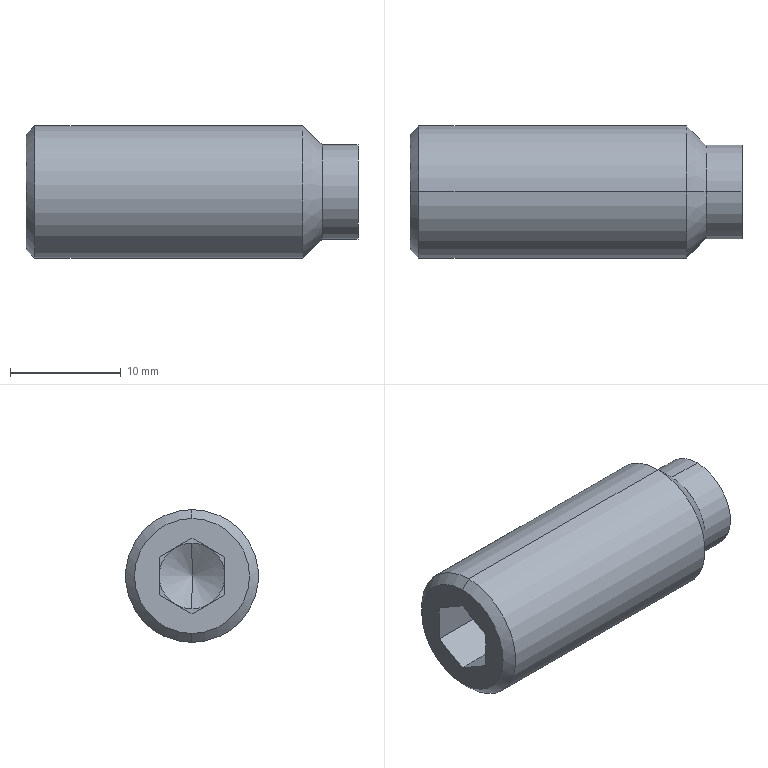Part | SolidWorks | features RevCut 2, Cut 1, LPattern 1, Revolution 1 | 1 solid | 24 faces | box 30 x 12 x 12 mm | volume 2983 mm3 | plane 14 | cone 6 | cylinder 4 | commonest cylinder face diameters 8.5 x2 12 x2
STEP:
#1=CARTESIAN_POINT('',(6.515,0.,0.));
#2=VERTEX_POINT('',#1);
#3=CARTESIAN_POINT('',(4.8,0.,2.97));
#4=VERTEX_POINT('',#3);
#5=CARTESIAN_POINT('',(6.515,0.,0.));
#6=DIRECTION('',(-0.5,0.,0.866));
#7=VECTOR('',#6,1000.);
#8=LINE('',#5,#7);
#9=EDGE_CURVE('',#2,#4,#8,.T.);
#10=ORIENTED_EDGE('',*,*,#9,.F.);
#11=CARTESIAN_POINT('',(4.8,0.,-2.97));
#12=VERTEX_POINT('',#11);
#13=CARTESIAN_POINT('',(6.515,0.,0.));
#14=DIRECTION('',(-0.5,0.,-0.866));
#15=VECTOR('',#14,1000.);
#16=LINE('',#13,#15);
#17=EDGE_CURVE('',#2,#12,#16,.T.);
#18=ORIENTED_EDGE('',*,*,#17,.T.);
#19=CARTESIAN_POINT('',(4.8,-1.485,-2.573));
#20=VERTEX_POINT('',#19);
#21=CARTESIAN_POINT('',(4.8,0.,0.));
#22=DIRECTION('',(-1.,0.,0.));
#23=DIRECTION('',(0.,0.,1.));
#24=AXIS2_PLACEMENT_3D('',#21,#22,#23);
#25=CIRCLE('',#24,2.97);
#26=EDGE_CURVE('',#12,#20,#25,.T.);
#27=ORIENTED_EDGE('',*,*,#26,.T.);
#28=CARTESIAN_POINT('',(4.8,-2.97,0.));
#29=VERTEX_POINT('',#28);
#30=CARTESIAN_POINT('',(4.8,0.,0.));
#31=DIRECTION('',(-1.,0.,0.));
#32=DIRECTION('',(0.,0.,1.));
#33=AXIS2_PLACEMENT_3D('',#30,#31,#32);
#34=CIRCLE('',#33,2.97);
#35=EDGE_CURVE('',#20,#29,#34,.T.);
#36=ORIENTED_EDGE('',*,*,#35,.T.);
#37=CARTESIAN_POINT('',(4.8,-1.485,2.573));
#38=VERTEX_POINT('',#37);
#39=CARTESIAN_POINT('',(4.8,0.,0.));
#40=DIRECTION('',(-1.,0.,0.));
#41=DIRECTION('',(0.,0.,1.));
#42=AXIS2_PLACEMENT_3D('',#39,#40,#41);
#43=CIRCLE('',#42,2.97);
#44=EDGE_CURVE('',#29,#38,#43,.T.);
#45=ORIENTED_EDGE('',*,*,#44,.T.);
#46=CARTESIAN_POINT('',(4.8,0.,0.));
#47=DIRECTION('',(-1.,0.,0.));
#48=DIRECTION('',(0.,0.,1.));
#49=AXIS2_PLACEMENT_3D('',#46,#47,#48);
#50=CIRCLE('',#49,2.97);
#51=EDGE_CURVE('',#38,#4,#50,.T.);
#52=ORIENTED_EDGE('',*,*,#51,.T.);
#53=EDGE_LOOP('',(#10,#18,#27,#36,#45,#52));
#54=FACE_OUTER_BOUND('',#53,.T.);
#55=CARTESIAN_POINT('',(-993.485,0.,0.));
#56=DIRECTION('',(-1.,0.,0.));
#57=DIRECTION('',(0.,0.,1.));
#58=AXIS2_PLACEMENT_3D('',#55,#56,#57);
#59=CONICAL_SURFACE('',#58,1732.051,1.047);
#60=ADVANCED_FACE('',(#54),#59,.F.);
#61=CARTESIAN_POINT('',(0.,0.,5.196));
#62=VERTEX_POINT('',#61);
#63=CARTESIAN_POINT('',(0.,0.,-5.196));
#64=VERTEX_POINT('',#63);
#65=CARTESIAN_POINT('',(0.,0.,0.));
#66=DIRECTION('',(-1.,0.,0.));
#67=DIRECTION('',(0.,0.,1.));
#68=AXIS2_PLACEMENT_3D('',#65,#66,#67);
#69=CIRCLE('',#68,5.196);
#70=EDGE_CURVE('',#62,#64,#69,.T.);
#71=ORIENTED_EDGE('',*,*,#70,.F.);
#72=CARTESIAN_POINT('',(0.804,0.,6.));
#73=VERTEX_POINT('',#72);
#74=CARTESIAN_POINT('',(0.804,0.,6.));
#75=DIRECTION('',(0.7071,0.,0.7071));
#76=VECTOR('',#75,1000.);
#77=LINE('',#74,#76);
#78=EDGE_CURVE('',#62,#73,#77,.T.);
#79=ORIENTED_EDGE('',*,*,#78,.T.);
#80=CARTESIAN_POINT('',(0.804,0.,-6.));
#81=VERTEX_POINT('',#80);
#82=CARTESIAN_POINT('',(0.804,0.,0.));
#83=DIRECTION('',(-1.,0.,0.));
#84=DIRECTION('',(0.,0.,1.));
#85=AXIS2_PLACEMENT_3D('',#82,#83,#84);
#86=CIRCLE('',#85,6.);
#87=EDGE_CURVE('',#73,#81,#86,.T.);
#88=ORIENTED_EDGE('',*,*,#87,.T.);
#89=CARTESIAN_POINT('',(0.804,0.,-6.));
#90=DIRECTION('',(0.7071,0.,-0.7071));
#91=VECTOR('',#90,1000.);
#92=LINE('',#89,#91);
#93=EDGE_CURVE('',#64,#81,#92,.T.);
#94=ORIENTED_EDGE('',*,*,#93,.F.);
#95=EDGE_LOOP('',(#71,#79,#88,#94));
#96=FACE_OUTER_BOUND('',#95,.T.);
#97=CARTESIAN_POINT('',(0.804,0.,0.));
#98=DIRECTION('',(1.,0.,0.));
#99=DIRECTION('',(0.,0.,-1.));
#100=AXIS2_PLACEMENT_3D('',#97,#98,#99);
#101=CONICAL_SURFACE('',#100,6.,0.7854);
#102=ADVANCED_FACE('',(#96),#101,.T.);
#103=CARTESIAN_POINT('',(25.,0.,6.));
#104=VERTEX_POINT('',#103);
#105=CARTESIAN_POINT('',(25.,0.,-6.));
#106=VERTEX_POINT('',#105);
#107=CARTESIAN_POINT('',(25.,0.,0.));
#108=DIRECTION('',(-1.,0.,0.));
#109=DIRECTION('',(0.,0.,1.));
#110=AXIS2_PLACEMENT_3D('',#107,#108,#109);
#111=CIRCLE('',#110,6.);
#112=EDGE_CURVE('',#104,#106,#111,.T.);
#113=ORIENTED_EDGE('',*,*,#112,.T.);
#114=CARTESIAN_POINT('',(-0.6655,0.,-6.));
#115=DIRECTION('',(-1.,0.,0.));
#116=VECTOR('',#115,1000.);
#117=LINE('',#114,#116);
#118=EDGE_CURVE('',#106,#81,#117,.T.);
#119=ORIENTED_EDGE('',*,*,#118,.T.);
#120=ORIENTED_EDGE('',*,*,#87,.F.);
#121=CARTESIAN_POINT('',(-0.6655,0.,6.));
#122=DIRECTION('',(-1.,0.,0.));
#123=VECTOR('',#122,1000.);
#124=LINE('',#121,#123);
#125=EDGE_CURVE('',#104,#73,#124,.T.);
#126=ORIENTED_EDGE('',*,*,#125,.F.);
#127=EDGE_LOOP('',(#113,#119,#120,#126));
#128=FACE_OUTER_BOUND('',#127,.T.);
#129=CARTESIAN_POINT('',(-0.6655,0.,0.));
#130=DIRECTION('',(-1.,0.,0.));
#131=DIRECTION('',(0.,0.,1.));
#132=AXIS2_PLACEMENT_3D('',#129,#130,#131);
#133=CYLINDRICAL_SURFACE('',#132,6.);
#134=ADVANCED_FACE('',(#128),#133,.T.);
#135=CARTESIAN_POINT('',(26.75,0.,4.25));
#136=VERTEX_POINT('',#135);
#137=CARTESIAN_POINT('',(26.75,0.,-4.25));
#138=VERTEX_POINT('',#137);
#139=CARTESIAN_POINT('',(26.75,0.,0.));
#140=DIRECTION('',(-1.,0.,0.));
#141=DIRECTION('',(0.,0.,1.));
#142=AXIS2_PLACEMENT_3D('',#139,#140,#141);
#143=CIRCLE('',#142,4.25);
#144=EDGE_CURVE('',#136,#138,#143,.T.);
#145=ORIENTED_EDGE('',*,*,#144,.T.);
#146=CARTESIAN_POINT('',(26.75,0.,-4.25));
#147=DIRECTION('',(-0.7071,0.,-0.7071));
#148=VECTOR('',#147,1000.);
#149=LINE('',#146,#148);
#150=EDGE_CURVE('',#138,#106,#149,.T.);
#151=ORIENTED_EDGE('',*,*,#150,.T.);
#152=ORIENTED_EDGE('',*,*,#112,.F.);
#153=CARTESIAN_POINT('',(26.75,0.,4.25));
#154=DIRECTION('',(-0.7071,0.,0.7071));
#155=VECTOR('',#154,1000.);
#156=LINE('',#153,#155);
#157=EDGE_CURVE('',#136,#104,#156,.T.);
#158=ORIENTED_EDGE('',*,*,#157,.F.);
#159=EDGE_LOOP('',(#145,#151,#152,#158));
#160=FACE_OUTER_BOUND('',#159,.T.);
#161=CARTESIAN_POINT('',(26.75,0.,0.));
#162=DIRECTION('',(-1.,0.,0.));
#163=DIRECTION('',(0.,0.,1.));
#164=AXIS2_PLACEMENT_3D('',#161,#162,#163);
#165=CONICAL_SURFACE('',#164,4.25,0.7854);
#166=ADVANCED_FACE('',(#160),#165,.T.);
#167=CARTESIAN_POINT('',(30.,0.,4.25));
#168=VERTEX_POINT('',#167);
#169=CARTESIAN_POINT('',(30.,0.,-4.25));
#170=VERTEX_POINT('',#169);
#171=CARTESIAN_POINT('',(30.,0.,0.));
#172=DIRECTION('',(-1.,0.,0.));
#173=DIRECTION('',(0.,0.,1.));
#174=AXIS2_PLACEMENT_3D('',#171,#172,#173);
#175=CIRCLE('',#174,4.25);
#176=EDGE_CURVE('',#168,#170,#175,.T.);
#177=ORIENTED_EDGE('',*,*,#176,.T.);
#178=CARTESIAN_POINT('',(-0.6655,0.,-4.25));
#179=DIRECTION('',(-1.,0.,0.));
#180=VECTOR('',#179,1000.);
#181=LINE('',#178,#180);
#182=EDGE_CURVE('',#170,#138,#181,.T.);
#183=ORIENTED_EDGE('',*,*,#182,.T.);
#184=ORIENTED_EDGE('',*,*,#144,.F.);
#185=CARTESIAN_POINT('',(-0.6655,0.,4.25));
#186=DIRECTION('',(-1.,0.,0.));
#187=VECTOR('',#186,1000.);
#188=LINE('',#185,#187);
#189=EDGE_CURVE('',#168,#136,#188,.T.);
#190=ORIENTED_EDGE('',*,*,#189,.F.);
#191=EDGE_LOOP('',(#177,#183,#184,#190));
#192=FACE_OUTER_BOUND('',#191,.T.);
#193=CARTESIAN_POINT('',(-0.6655,0.,0.));
#194=DIRECTION('',(-1.,0.,0.));
#195=DIRECTION('',(0.,0.,1.));
#196=AXIS2_PLACEMENT_3D('',#193,#194,#195);
#197=CYLINDRICAL_SURFACE('',#196,4.25);
#198=ADVANCED_FACE('',(#192),#197,.T.);
#199=CARTESIAN_POINT('',(4.8,1.485,2.573));
#200=VERTEX_POINT('',#199);
#201=CARTESIAN_POINT('',(4.8,2.97,0.));
#202=VERTEX_POINT('',#201);
#203=CARTESIAN_POINT('',(4.8,0.,0.));
#204=DIRECTION('',(-1.,0.,0.));
#205=DIRECTION('',(0.,0.,1.));
#206=AXIS2_PLACEMENT_3D('',#203,#204,#205);
#207=CIRCLE('',#206,2.97);
#208=EDGE_CURVE('',#200,#202,#207,.T.);
#209=ORIENTED_EDGE('',*,*,#208,.F.);
#210=CARTESIAN_POINT('',(4.8,2.97,1.715));
#211=VERTEX_POINT('',#210);
#212=CARTESIAN_POINT('',(4.8,0.,3.43));
#213=DIRECTION('',(0.,0.866,-0.5));
#214=VECTOR('',#213,1000.);
#215=LINE('',#212,#214);
#216=EDGE_CURVE('',#200,#211,#215,.T.);
#217=ORIENTED_EDGE('',*,*,#216,.T.);
#218=CARTESIAN_POINT('',(4.8,2.97,1.715));
#219=DIRECTION('',(0.,0.,-1.));
#220=VECTOR('',#219,1000.);
#221=LINE('',#218,#220);
#222=EDGE_CURVE('',#211,#202,#221,.T.);
#223=ORIENTED_EDGE('',*,*,#222,.T.);
#224=EDGE_LOOP('',(#209,#217,#223));
#225=FACE_OUTER_BOUND('',#224,.T.);
#226=CARTESIAN_POINT('',(4.8,2.97,5.145));
#227=DIRECTION('',(-1.,0.,0.));
#228=DIRECTION('',(0.,0.,1.));
#229=AXIS2_PLACEMENT_3D('',#226,#227,#228);
#230=PLANE('',#229);
#231=ADVANCED_FACE('',(#225),#230,.T.);
#232=CARTESIAN_POINT('',(4.8,1.485,-2.573));
#233=VERTEX_POINT('',#232);
#234=CARTESIAN_POINT('',(4.8,0.,0.));
#235=DIRECTION('',(-1.,0.,0.));
#236=DIRECTION('',(0.,0.,1.));
#237=AXIS2_PLACEMENT_3D('',#234,#235,#236);
#238=CIRCLE('',#237,2.97);
#239=EDGE_CURVE('',#202,#233,#238,.T.);
#240=ORIENTED_EDGE('',*,*,#239,.F.);
#241=CARTESIAN_POINT('',(4.8,2.97,-1.715));
#242=VERTEX_POINT('',#241);
#243=CARTESIAN_POINT('',(4.8,2.97,1.715));
#244=DIRECTION('',(0.,0.,-1.));
#245=VECTOR('',#244,1000.);
#246=LINE('',#243,#245);
#247=EDGE_CURVE('',#202,#242,#246,.T.);
#248=ORIENTED_EDGE('',*,*,#247,.T.);
#249=CARTESIAN_POINT('',(4.8,2.97,-1.715));
#250=DIRECTION('',(0.,-0.866,-0.5));
#251=VECTOR('',#250,1000.);
#252=LINE('',#249,#251);
#253=EDGE_CURVE('',#242,#233,#252,.T.);
#254=ORIENTED_EDGE('',*,*,#253,.T.);
#255=EDGE_LOOP('',(#240,#248,#254));
#256=FACE_OUTER_BOUND('',#255,.T.);
#257=CARTESIAN_POINT('',(4.8,2.97,5.145));
#258=DIRECTION('',(-1.,0.,0.));
#259=DIRECTION('',(0.,0.,1.));
#260=AXIS2_PLACEMENT_3D('',#257,#258,#259);
#261=PLANE('',#260);
#262=ADVANCED_FACE('',(#256),#261,.T.);
#263=CARTESIAN_POINT('',(4.8,0.,0.));
#264=DIRECTION('',(-1.,0.,0.));
#265=DIRECTION('',(0.,0.,1.));
#266=AXIS2_PLACEMENT_3D('',#263,#264,#265);
#267=CIRCLE('',#266,2.97);
#268=EDGE_CURVE('',#233,#12,#267,.T.);
#269=ORIENTED_EDGE('',*,*,#268,.F.);
#270=CARTESIAN_POINT('',(4.8,0.,-3.43));
#271=VERTEX_POINT('',#270);
#272=CARTESIAN_POINT('',(4.8,2.97,-1.715));
#273=DIRECTION('',(0.,-0.866,-0.5));
#274=VECTOR('',#273,1000.);
#275=LINE('',#272,#274);
#276=EDGE_CURVE('',#233,#271,#275,.T.);
#277=ORIENTED_EDGE('',*,*,#276,.T.);
#278=CARTESIAN_POINT('',(4.8,0.,-3.43));
#279=DIRECTION('',(0.,-0.866,0.5));
#280=VECTOR('',#279,1000.);
#281=LINE('',#278,#280);
#282=EDGE_CURVE('',#271,#20,#281,.T.);
#283=ORIENTED_EDGE('',*,*,#282,.T.);
#284=ORIENTED_EDGE('',*,*,#26,.F.);
#285=EDGE_LOOP('',(#269,#277,#283,#284));
#286=FACE_OUTER_BOUND('',#285,.T.);
#287=CARTESIAN_POINT('',(4.8,2.97,5.145));
#288=DIRECTION('',(-1.,0.,0.));
#289=DIRECTION('',(0.,0.,1.));
#290=AXIS2_PLACEMENT_3D('',#287,#288,#289);
#291=PLANE('',#290);
#292=ADVANCED_FACE('',(#286),#291,.T.);
#293=ORIENTED_EDGE('',*,*,#35,.F.);
#294=CARTESIAN_POINT('',(4.8,-2.97,-1.715));
#295=VERTEX_POINT('',#294);
#296=CARTESIAN_POINT('',(4.8,0.,-3.43));
#297=DIRECTION('',(0.,-0.866,0.5));
#298=VECTOR('',#297,1000.);
#299=LINE('',#296,#298);
#300=EDGE_CURVE('',#20,#295,#299,.T.);
#301=ORIENTED_EDGE('',*,*,#300,.T.);
#302=CARTESIAN_POINT('',(4.8,-2.97,-1.715));
#303=DIRECTION('',(0.,0.,1.));
#304=VECTOR('',#303,1000.);
#305=LINE('',#302,#304);
#306=EDGE_CURVE('',#295,#29,#305,.T.);
#307=ORIENTED_EDGE('',*,*,#306,.T.);
#308=EDGE_LOOP('',(#293,#301,#307));
#309=FACE_OUTER_BOUND('',#308,.T.);
#310=CARTESIAN_POINT('',(4.8,2.97,5.145));
#311=DIRECTION('',(-1.,0.,0.));
#312=DIRECTION('',(0.,0.,1.));
#313=AXIS2_PLACEMENT_3D('',#310,#311,#312);
#314=PLANE('',#313);
#315=ADVANCED_FACE('',(#309),#314,.T.);
#316=ORIENTED_EDGE('',*,*,#44,.F.);
#317=CARTESIAN_POINT('',(4.8,-2.97,1.715));
#318=VERTEX_POINT('',#317);
#319=CARTESIAN_POINT('',(4.8,-2.97,-1.715));
#320=DIRECTION('',(0.,0.,1.));
#321=VECTOR('',#320,1000.);
#322=LINE('',#319,#321);
#323=EDGE_CURVE('',#29,#318,#322,.T.);
#324=ORIENTED_EDGE('',*,*,#323,.T.);
#325=CARTESIAN_POINT('',(4.8,-2.97,1.715));
#326=DIRECTION('',(0.,0.866,0.5));
#327=VECTOR('',#326,1000.);
#328=LINE('',#325,#327);
#329=EDGE_CURVE('',#318,#38,#328,.T.);
#330=ORIENTED_EDGE('',*,*,#329,.T.);
#331=EDGE_LOOP('',(#316,#324,#330));
#332=FACE_OUTER_BOUND('',#331,.T.);
#333=CARTESIAN_POINT('',(4.8,2.97,5.145));
#334=DIRECTION('',(-1.,0.,0.));
#335=DIRECTION('',(0.,0.,1.));
#336=AXIS2_PLACEMENT_3D('',#333,#334,#335);
#337=PLANE('',#336);
#338=ADVANCED_FACE('',(#332),#337,.T.);
#339=CARTESIAN_POINT('',(0.,0.,3.43));
#340=VERTEX_POINT('',#339);
#341=CARTESIAN_POINT('',(0.,2.97,1.715));
#342=VERTEX_POINT('',#341);
#343=CARTESIAN_POINT('',(0.,0.,3.43));
#344=DIRECTION('',(0.,0.866,-0.5));
#345=VECTOR('',#344,1000.);
#346=LINE('',#343,#345);
#347=EDGE_CURVE('',#340,#342,#346,.T.);
#348=ORIENTED_EDGE('',*,*,#347,.F.);
#349=CARTESIAN_POINT('',(0.,-2.97,1.715));
#350=VERTEX_POINT('',#349);
#351=CARTESIAN_POINT('',(0.,-2.97,1.715));
#352=DIRECTION('',(0.,0.866,0.5));
#353=VECTOR('',#352,1000.);
#354=LINE('',#351,#353);
#355=EDGE_CURVE('',#350,#340,#354,.T.);
#356=ORIENTED_EDGE('',*,*,#355,.F.);
#357=CARTESIAN_POINT('',(0.,-2.97,-1.715));
#358=VERTEX_POINT('',#357);
#359=CARTESIAN_POINT('',(0.,-2.97,-1.715));
#360=DIRECTION('',(0.,0.,1.));
#361=VECTOR('',#360,1000.);
#362=LINE('',#359,#361);
#363=EDGE_CURVE('',#358,#350,#362,.T.);
#364=ORIENTED_EDGE('',*,*,#363,.F.);
#365=CARTESIAN_POINT('',(0.,0.,-3.43));
#366=VERTEX_POINT('',#365);
#367=CARTESIAN_POINT('',(0.,0.,-3.43));
#368=DIRECTION('',(0.,-0.866,0.5));
#369=VECTOR('',#368,1000.);
#370=LINE('',#367,#369);
#371=EDGE_CURVE('',#366,#358,#370,.T.);
#372=ORIENTED_EDGE('',*,*,#371,.F.);
#373=CARTESIAN_POINT('',(0.,2.97,-1.715));
#374=VERTEX_POINT('',#373);
#375=CARTESIAN_POINT('',(0.,2.97,-1.715));
#376=DIRECTION('',(0.,-0.866,-0.5));
#377=VECTOR('',#376,1000.);
#378=LINE('',#375,#377);
#379=EDGE_CURVE('',#374,#366,#378,.T.);
#380=ORIENTED_EDGE('',*,*,#379,.F.);
#381=CARTESIAN_POINT('',(0.,2.97,1.715));
#382=DIRECTION('',(0.,0.,-1.));
#383=VECTOR('',#382,1000.);
#384=LINE('',#381,#383);
#385=EDGE_CURVE('',#342,#374,#384,.T.);
#386=ORIENTED_EDGE('',*,*,#385,.F.);
#387=EDGE_LOOP('',(#348,#356,#364,#372,#380,#386));
#388=FACE_BOUND('',#387,.T.);
#389=CARTESIAN_POINT('',(0.,0.,0.));
#390=DIRECTION('',(-1.,0.,0.));
#391=DIRECTION('',(0.,0.,1.));
#392=AXIS2_PLACEMENT_3D('',#389,#390,#391);
#393=CIRCLE('',#392,5.196);
#394=EDGE_CURVE('',#64,#62,#393,.T.);
#395=ORIENTED_EDGE('',*,*,#394,.T.);
#396=ORIENTED_EDGE('',*,*,#70,.T.);
#397=EDGE_LOOP('',(#395,#396));
#398=FACE_OUTER_BOUND('',#397,.T.);
#399=CARTESIAN_POINT('',(0.,5.196,0.));
#400=DIRECTION('',(1.,0.,0.));
#401=DIRECTION('',(0.,0.,-1.));
#402=AXIS2_PLACEMENT_3D('',#399,#400,#401);
#403=PLANE('',#402);
#404=ADVANCED_FACE('',(#388,#398),#403,.F.);
#405=ORIENTED_EDGE('',*,*,#176,.F.);
#406=CARTESIAN_POINT('',(30.,0.,0.));
#407=DIRECTION('',(-1.,0.,0.));
#408=DIRECTION('',(0.,0.,1.));
#409=AXIS2_PLACEMENT_3D('',#406,#407,#408);
#410=CIRCLE('',#409,4.25);
#411=EDGE_CURVE('',#170,#168,#410,.T.);
#412=ORIENTED_EDGE('',*,*,#411,.F.);
#413=EDGE_LOOP('',(#405,#412));
#414=FACE_OUTER_BOUND('',#413,.T.);
#415=CARTESIAN_POINT('',(30.,0.,0.));
#416=DIRECTION('',(-1.,0.,0.));
#417=DIRECTION('',(0.,0.,1.));
#418=AXIS2_PLACEMENT_3D('',#415,#416,#417);
#419=PLANE('',#418);
#420=ADVANCED_FACE('',(#414),#419,.F.);
#421=ORIENTED_EDGE('',*,*,#182,.F.);
#422=ORIENTED_EDGE('',*,*,#411,.T.);
#423=ORIENTED_EDGE('',*,*,#189,.T.);
#424=CARTESIAN_POINT('',(26.75,0.,0.));
#425=DIRECTION('',(-1.,0.,0.));
#426=DIRECTION('',(0.,0.,1.));
#427=AXIS2_PLACEMENT_3D('',#424,#425,#426);
#428=CIRCLE('',#427,4.25);
#429=EDGE_CURVE('',#138,#136,#428,.T.);
#430=ORIENTED_EDGE('',*,*,#429,.F.);
#431=EDGE_LOOP('',(#421,#422,#423,#430));
#432=FACE_OUTER_BOUND('',#431,.T.);
#433=CARTESIAN_POINT('',(-0.6655,0.,0.));
#434=DIRECTION('',(-1.,0.,0.));
#435=DIRECTION('',(0.,0.,1.));
#436=AXIS2_PLACEMENT_3D('',#433,#434,#435);
#437=CYLINDRICAL_SURFACE('',#436,4.25);
#438=ADVANCED_FACE('',(#432),#437,.T.);
#439=ORIENTED_EDGE('',*,*,#150,.F.);
#440=ORIENTED_EDGE('',*,*,#429,.T.);
#441=ORIENTED_EDGE('',*,*,#157,.T.);
#442=CARTESIAN_POINT('',(25.,0.,0.));
#443=DIRECTION('',(-1.,0.,0.));
#444=DIRECTION('',(0.,0.,1.));
#445=AXIS2_PLACEMENT_3D('',#442,#443,#444);
#446=CIRCLE('',#445,6.);
#447=EDGE_CURVE('',#106,#104,#446,.T.);
#448=ORIENTED_EDGE('',*,*,#447,.F.);
#449=EDGE_LOOP('',(#439,#440,#441,#448));
#450=FACE_OUTER_BOUND('',#449,.T.);
#451=CARTESIAN_POINT('',(26.75,0.,0.));
#452=DIRECTION('',(-1.,0.,0.));
#453=DIRECTION('',(0.,0.,1.));
#454=AXIS2_PLACEMENT_3D('',#451,#452,#453);
#455=CONICAL_SURFACE('',#454,4.25,0.7854);
#456=ADVANCED_FACE('',(#450),#455,.T.);
#457=ORIENTED_EDGE('',*,*,#118,.F.);
#458=ORIENTED_EDGE('',*,*,#447,.T.);
#459=ORIENTED_EDGE('',*,*,#125,.T.);
#460=CARTESIAN_POINT('',(0.804,0.,0.));
#461=DIRECTION('',(-1.,0.,0.));
#462=DIRECTION('',(0.,0.,1.));
#463=AXIS2_PLACEMENT_3D('',#460,#461,#462);
#464=CIRCLE('',#463,6.);
#465=EDGE_CURVE('',#81,#73,#464,.T.);
#466=ORIENTED_EDGE('',*,*,#465,.F.);
#467=EDGE_LOOP('',(#457,#458,#459,#466));
#468=FACE_OUTER_BOUND('',#467,.T.);
#469=CARTESIAN_POINT('',(-0.6655,0.,0.));
#470=DIRECTION('',(-1.,0.,0.));
#471=DIRECTION('',(0.,0.,1.));
#472=AXIS2_PLACEMENT_3D('',#469,#470,#471);
#473=CYLINDRICAL_SURFACE('',#472,6.);
#474=ADVANCED_FACE('',(#468),#473,.T.);
#475=ORIENTED_EDGE('',*,*,#78,.F.);
#476=ORIENTED_EDGE('',*,*,#394,.F.);
#477=ORIENTED_EDGE('',*,*,#93,.T.);
#478=ORIENTED_EDGE('',*,*,#465,.T.);
#479=EDGE_LOOP('',(#475,#476,#477,#478));
#480=FACE_OUTER_BOUND('',#479,.T.);
#481=CARTESIAN_POINT('',(0.804,0.,0.));
#482=DIRECTION('',(1.,0.,0.));
#483=DIRECTION('',(0.,0.,-1.));
#484=AXIS2_PLACEMENT_3D('',#481,#482,#483);
#485=CONICAL_SURFACE('',#484,6.,0.7854);
#486=ADVANCED_FACE('',(#480),#485,.T.);
#487=ORIENTED_EDGE('',*,*,#355,.T.);
#488=CARTESIAN_POINT('',(4.8,0.,3.43));
#489=VERTEX_POINT('',#488);
#490=CARTESIAN_POINT('',(4.8,0.,3.43));
#491=DIRECTION('',(-1.,0.,0.));
#492=VECTOR('',#491,1000.);
#493=LINE('',#490,#492);
#494=EDGE_CURVE('',#489,#340,#493,.T.);
#495=ORIENTED_EDGE('',*,*,#494,.F.);
#496=CARTESIAN_POINT('',(4.8,-2.97,1.715));
#497=DIRECTION('',(0.,0.866,0.5));
#498=VECTOR('',#497,1000.);
#499=LINE('',#496,#498);
#500=EDGE_CURVE('',#38,#489,#499,.T.);
#501=ORIENTED_EDGE('',*,*,#500,.F.);
#502=ORIENTED_EDGE('',*,*,#329,.F.);
#503=CARTESIAN_POINT('',(4.8,-2.97,1.715));
#504=DIRECTION('',(-1.,0.,0.));
#505=VECTOR('',#504,1000.);
#506=LINE('',#503,#505);
#507=EDGE_CURVE('',#318,#350,#506,.T.);
#508=ORIENTED_EDGE('',*,*,#507,.T.);
#509=EDGE_LOOP('',(#487,#495,#501,#502,#508));
#510=FACE_OUTER_BOUND('',#509,.T.);
#511=CARTESIAN_POINT('',(4.8,-2.97,1.715));
#512=DIRECTION('',(0.,-0.5,0.866));
#513=DIRECTION('',(0.,-0.866,-0.5));
#514=AXIS2_PLACEMENT_3D('',#511,#512,#513);
#515=PLANE('',#514);
#516=ADVANCED_FACE('',(#510),#515,.F.);
#517=ORIENTED_EDGE('',*,*,#363,.T.);
#518=ORIENTED_EDGE('',*,*,#507,.F.);
#519=ORIENTED_EDGE('',*,*,#323,.F.);
#520=ORIENTED_EDGE('',*,*,#306,.F.);
#521=CARTESIAN_POINT('',(4.8,-2.97,-1.715));
#522=DIRECTION('',(-1.,0.,0.));
#523=VECTOR('',#522,1000.);
#524=LINE('',#521,#523);
#525=EDGE_CURVE('',#295,#358,#524,.T.);
#526=ORIENTED_EDGE('',*,*,#525,.T.);
#527=EDGE_LOOP('',(#517,#518,#519,#520,#526));
#528=FACE_OUTER_BOUND('',#527,.T.);
#529=CARTESIAN_POINT('',(4.8,-2.97,-1.715));
#530=DIRECTION('',(0.,-1.,0.));
#531=DIRECTION('',(0.,0.,-1.));
#532=AXIS2_PLACEMENT_3D('',#529,#530,#531);
#533=PLANE('',#532);
#534=ADVANCED_FACE('',(#528),#533,.F.);
#535=ORIENTED_EDGE('',*,*,#371,.T.);
#536=ORIENTED_EDGE('',*,*,#525,.F.);
#537=ORIENTED_EDGE('',*,*,#300,.F.);
#538=ORIENTED_EDGE('',*,*,#282,.F.);
#539=CARTESIAN_POINT('',(4.8,0.,-3.43));
#540=DIRECTION('',(-1.,0.,0.));
#541=VECTOR('',#540,1000.);
#542=LINE('',#539,#541);
#543=EDGE_CURVE('',#271,#366,#542,.T.);
#544=ORIENTED_EDGE('',*,*,#543,.T.);
#545=EDGE_LOOP('',(#535,#536,#537,#538,#544));
#546=FACE_OUTER_BOUND('',#545,.T.);
#547=CARTESIAN_POINT('',(4.8,0.,-3.43));
#548=DIRECTION('',(0.,-0.5,-0.866));
#549=DIRECTION('',(0.,0.866,-0.5));
#550=AXIS2_PLACEMENT_3D('',#547,#548,#549);
#551=PLANE('',#550);
#552=ADVANCED_FACE('',(#546),#551,.F.);
#553=ORIENTED_EDGE('',*,*,#379,.T.);
#554=ORIENTED_EDGE('',*,*,#543,.F.);
#555=ORIENTED_EDGE('',*,*,#276,.F.);
#556=ORIENTED_EDGE('',*,*,#253,.F.);
#557=CARTESIAN_POINT('',(4.8,2.97,-1.715));
#558=DIRECTION('',(-1.,0.,0.));
#559=VECTOR('',#558,1000.);
#560=LINE('',#557,#559);
#561=EDGE_CURVE('',#242,#374,#560,.T.);
#562=ORIENTED_EDGE('',*,*,#561,.T.);
#563=EDGE_LOOP('',(#553,#554,#555,#556,#562));
#564=FACE_OUTER_BOUND('',#563,.T.);
#565=CARTESIAN_POINT('',(4.8,2.97,-1.715));
#566=DIRECTION('',(0.,0.5,-0.866));
#567=DIRECTION('',(0.,0.866,0.5));
#568=AXIS2_PLACEMENT_3D('',#565,#566,#567);
#569=PLANE('',#568);
#570=ADVANCED_FACE('',(#564),#569,.F.);
#571=ORIENTED_EDGE('',*,*,#385,.T.);
#572=ORIENTED_EDGE('',*,*,#561,.F.);
#573=ORIENTED_EDGE('',*,*,#247,.F.);
#574=ORIENTED_EDGE('',*,*,#222,.F.);
#575=CARTESIAN_POINT('',(4.8,2.97,1.715));
#576=DIRECTION('',(-1.,0.,0.));
#577=VECTOR('',#576,1000.);
#578=LINE('',#575,#577);
#579=EDGE_CURVE('',#211,#342,#578,.T.);
#580=ORIENTED_EDGE('',*,*,#579,.T.);
#581=EDGE_LOOP('',(#571,#572,#573,#574,#580));
#582=FACE_OUTER_BOUND('',#581,.T.);
#583=CARTESIAN_POINT('',(4.8,2.97,1.715));
#584=DIRECTION('',(0.,1.,0.));
#585=DIRECTION('',(0.,0.,1.));
#586=AXIS2_PLACEMENT_3D('',#583,#584,#585);
#587=PLANE('',#586);
#588=ADVANCED_FACE('',(#582),#587,.F.);
#589=ORIENTED_EDGE('',*,*,#347,.T.);
#590=ORIENTED_EDGE('',*,*,#579,.F.);
#591=ORIENTED_EDGE('',*,*,#216,.F.);
#592=CARTESIAN_POINT('',(4.8,0.,3.43));
#593=DIRECTION('',(0.,0.866,-0.5));
#594=VECTOR('',#593,1000.);
#595=LINE('',#592,#594);
#596=EDGE_CURVE('',#489,#200,#595,.T.);
#597=ORIENTED_EDGE('',*,*,#596,.F.);
#598=ORIENTED_EDGE('',*,*,#494,.T.);
#599=EDGE_LOOP('',(#589,#590,#591,#597,#598));
#600=FACE_OUTER_BOUND('',#599,.T.);
#601=CARTESIAN_POINT('',(4.8,0.,3.43));
#602=DIRECTION('',(0.,0.5,0.866));
#603=DIRECTION('',(0.,-0.866,0.5));
#604=AXIS2_PLACEMENT_3D('',#601,#602,#603);
#605=PLANE('',#604);
#606=ADVANCED_FACE('',(#600),#605,.F.);
#607=ORIENTED_EDGE('',*,*,#51,.F.);
#608=ORIENTED_EDGE('',*,*,#500,.T.);
#609=ORIENTED_EDGE('',*,*,#596,.T.);
#610=CARTESIAN_POINT('',(4.8,0.,0.));
#611=DIRECTION('',(-1.,0.,0.));
#612=DIRECTION('',(0.,0.,1.));
#613=AXIS2_PLACEMENT_3D('',#610,#611,#612);
#614=CIRCLE('',#613,2.97);
#615=EDGE_CURVE('',#4,#200,#614,.T.);
#616=ORIENTED_EDGE('',*,*,#615,.F.);
#617=EDGE_LOOP('',(#607,#608,#609,#616));
#618=FACE_OUTER_BOUND('',#617,.T.);
#619=CARTESIAN_POINT('',(4.8,2.97,5.145));
#620=DIRECTION('',(-1.,0.,0.));
#621=DIRECTION('',(0.,0.,1.));
#622=AXIS2_PLACEMENT_3D('',#619,#620,#621);
#623=PLANE('',#622);
#624=ADVANCED_FACE('',(#618),#623,.T.);
#625=ORIENTED_EDGE('',*,*,#17,.F.);
#626=ORIENTED_EDGE('',*,*,#9,.T.);
#627=ORIENTED_EDGE('',*,*,#615,.T.);
#628=ORIENTED_EDGE('',*,*,#208,.T.);
#629=ORIENTED_EDGE('',*,*,#239,.T.);
#630=ORIENTED_EDGE('',*,*,#268,.T.);
#631=EDGE_LOOP('',(#625,#626,#627,#628,#629,#630));
#632=FACE_OUTER_BOUND('',#631,.T.);
#633=CARTESIAN_POINT('',(-993.485,0.,0.));
#634=DIRECTION('',(-1.,0.,0.));
#635=DIRECTION('',(0.,0.,1.));
#636=AXIS2_PLACEMENT_3D('',#633,#634,#635);
#637=CONICAL_SURFACE('',#636,1732.051,1.047);
#638=ADVANCED_FACE('',(#632),#637,.F.);
#639=CLOSED_SHELL('',(#60,#102,#134,#166,#198,#231,#262,#292,#315,#338,#404,#420,#438,#456,#474,#486,#516,#534,#552,#570,#588,#606,#624,#638));
#640=MANIFOLD_SOLID_BREP('',#639);
#641=CARTESIAN_POINT('',(0.,0.,0.));
#642=DIRECTION('',(0.,0.,1.));
#643=DIRECTION('',(1.,0.,0.));
#644=AXIS2_PLACEMENT_3D('',#641,#642,#643);
#645=(LENGTH_UNIT()NAMED_UNIT(*)SI_UNIT(.MILLI.,.METRE.));
#646=UNCERTAINTY_MEASURE_WITH_UNIT(LENGTH_MEASURE(0.00001),#645,'','');
#647=(NAMED_UNIT(*)PLANE_ANGLE_UNIT()SI_UNIT($,.RADIAN.));
#648=(NAMED_UNIT(*)SI_UNIT($,.STERADIAN.)SOLID_ANGLE_UNIT());
#649=(GEOMETRIC_REPRESENTATION_CONTEXT(3)GLOBAL_UNCERTAINTY_ASSIGNED_CONTEXT((#646))GLOBAL_UNIT_ASSIGNED_CONTEXT((#645,#647,#648))REPRESENTATION_CONTEXT('',''));
#650=ADVANCED_BREP_SHAPE_REPRESENTATION('',(#640,#644),#649);